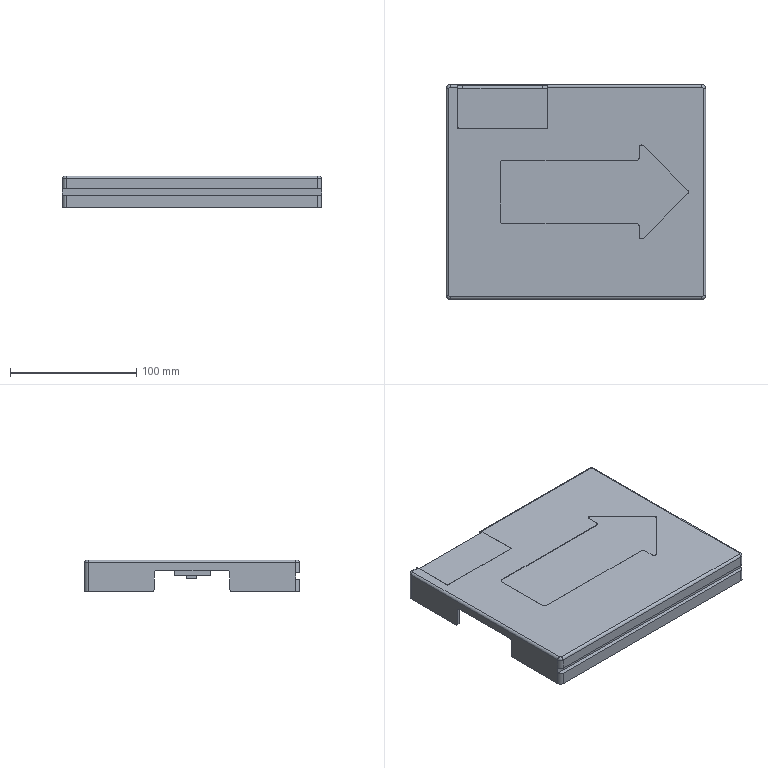NC program | NX | posted with a generic post | part box 205 x 170 x 25 mm
Lines 98 to 1305 of 17262:
(CAVITY_MILL_1 , TOOL : D10)
N188 T04 M6
N190 G54
N192 G17 G0 G90 X-109.497 Y-4.33 B0. C0. S9500 M3
N194 G43 Z30. H4
N196 Z0.513
N198 G94 G1 Z-0.988 F1000.
N200 X-103.497 Y-0.866
N202 G3 X-102.997 Y0. R1.
N204 G1 Y43.982 F3000.
N206 G2 X-103.677 Y44.075 R6.324
N208 G1 X-107.497
N210 Y45.275
N212 X-103.556
N214 G3 X-102.5 Y45.16 R5.124
N216 G1 X-100.5
N218 G3 X-95.4 Y50.272 R5.123
N220 G1 Y74.9
N222 X95.4
N224 Y30.272
N226 G3 X100.5 Y25.16 R5.125
N228 G1 X102.5
N230 G3 X103.55 Y25.275 R5.13
N232 G1 X107.497
N234 Y24.075
N236 X103.671
N238 G2 X102.997 Y23.982 R6.33
N240 G1 Y-23.982
N242 G2 X103.672 Y-24.075 R6.329
N244 G1 X107.497
N246 Y-25.275
N248 X103.551
N250 G3 X102.5 Y-25.16 R5.129
N252 G1 X100.5
N254 G3 X95.4 Y-30.272 R5.126
N256 G1 Y-68.9
N258 Y-74.9
N260 X-0.005
N262 X-95.4
N264 Y-50.272
N266 G3 X-100.5 Y-45.16 R5.106
N268 G1 X-102.5
N270 G3 X-103.558 Y-45.275 R5.122
N272 G1 X-107.497
N274 Y-44.075
N276 X-103.679
N278 G2 X-102.997 Y-43.982 R6.322
N280 G1 Y0.
N282 X-96.997
N284 Y39.734
N286 G3 X-89.4 Y50.266 R11.123
N288 G1 Y68.9
N290 X89.4
N292 Y30.265
N294 G3 X96.997 Y19.734 R11.125
N296 G1 Y-19.735
N298 G3 X89.4 Y-30.264 R11.126
N300 G1 Y-68.9
N302 X-89.4
N304 Y-50.276
N306 G3 X-96.997 Y-39.729 R11.106
N308 G1 Y0.
N310 X-90.997
N312 Y36.054
N314 G3 X-83.4 Y50.262 R17.123
N316 G1 Y62.9
N318 X83.4
N320 Y30.26
N322 G3 X90.997 Y16.055 R17.125
N324 G1 Y-16.056
N326 G3 X83.4 Y-30.258 R17.126
N328 G1 Y-62.9
N330 X-83.4
N332 Y-50.278
N334 G3 X-90.997 Y-36.047 R17.106
N336 G1 Y0.
N338 X-84.997
N340 Y33.148
N342 G3 X-77.4 Y50.258 R23.123
N344 G1 Y56.9
N346 X77.4
N348 Y30.256
N350 G3 X84.997 Y13.149 R23.125
N352 G1 Y-13.15
N354 G3 X77.4 Y-30.253 R23.126
N356 G1 Y-56.9
N358 X-77.4
N360 Y-50.28
N362 G3 X-84.997 Y-33.138 R23.106
N364 G1 Y0.
N366 X-78.997
N368 Y30.667
N370 G3 X-71.4 Y50.255 R29.123
N372 G1 Y50.9
N374 X71.4
N376 Y30.252
N378 G3 X78.997 Y10.668 R29.125
N380 G1 Y-10.669
N382 G3 X71.4 Y-30.249 R29.126
N384 G1 Y-50.9
N386 X-71.4
N388 Y-50.281
N390 G3 X-78.997 Y-30.657 R29.106
N392 G1 Y0.
N394 X-72.997
N396 Y28.467
N398 G3 X-65.815 Y44.9 R35.123
N400 G1 X65.4
N402 Y30.249
N404 G3 X72.997 Y8.468 R35.125
N406 G1 Y-8.469
N408 G3 X65.4 Y-30.245 R35.126
N410 G1 Y-44.9
N412 X-65.813
N414 G3 X-72.997 Y-28.456 R35.106
N416 G1 Y0.
N418 X-66.997
N420 Y26.469
N422 G3 X-61.007 Y38.9 R41.123
N424 G1 X59.4
N426 Y30.243
N428 G3 X66.997 Y6.47 R41.125
N430 G1 Y-6.471
N432 G3 X59.4 Y-30.242 R41.126
N434 G1 Y-38.9
N436 X-61.003
N438 G3 X-66.997 Y-26.457 R41.106
N440 G1 Y0.
N442 X-60.997
N444 Y24.626
N446 G3 X-56.723 Y32.9 R47.123
N448 G1 X53.4
N450 Y30.236
N452 G3 X60.997 Y4.627 R47.125
N454 G1 Y-4.628
N456 G3 X53.4 Y-30.235 R47.126
N458 G1 Y-32.9
N460 X-56.718
N462 G3 X-60.997 Y-24.614 R47.106
N464 G1 Y0.
N466 X-54.997
N468 Y22.907
N470 G3 X-52.823 Y26.9 R53.123
N472 G1 X47.508
N474 G3 X54.997 Y2.908 R53.125
N476 G1 Y-2.909
N478 G3 X47.508 Y-26.9 R53.126
N480 G1 X-52.817
N482 G3 X-54.997 Y-22.895 R53.106
N484 G1 Y0.
N486 X-48.997
N488 Y20.9
N490 X42.15
N492 G3 X48.997 Y1.291 R59.125
N494 G1 Y-1.292
N496 G3 X42.15 Y-20.9 R59.126
N498 G1 X-48.997
N500 Y0.
N502 X-42.997
N504 Y14.9
N506 X37.243
N508 G3 X42.87 Y-0.001 R65.125
N510 X37.244 Y-14.9 R65.126
N512 G1 X-42.997
N514 Y0.
N516 X-36.997
N518 Y8.9
N520 X32.691
N522 G3 X36.17 Y-0.001 R71.125
N524 X32.691 Y-8.9 R71.126
N526 G1 X-36.997
N528 Y0.
N530 X-30.997
N532 Y2.9
N534 X28.425
N536 G3 X29.595 Y-0.001 R77.125
N538 X28.426 Y-2.9 R77.126
N540 G1 X-30.997
N542 Y0.
N544 G3 X-31.497 Y0.866 R1.
N546 G1 Z0.513
N548 G0 X-109.497 Y-4.33 Z-0.475
N550 G1 Z-1.975 F1000.
N552 X-103.497 Y-0.866
N554 G3 X-102.997 Y0. R1.
N556 G1 Y43.729 F3000.
N558 G2 X-103.58 Y43.802 R6.284
N560 G1 X-107.497
N562 Y45.002
N564 X-103.472
N566 G3 X-102.861 Y44.923 R5.084
N568 X-100.151 Y44.92 R20.2
N570 X-95.4 Y49.997 R5.088
N572 G1 Y74.9
N574 X95.4
N576 Y29.995
N578 G3 X100.164 Y24.92 R5.085
N580 X102.829 Y24.919 R21.254
N582 X103.477 Y25.002 R5.088
N584 G1 X107.497
N586 Y24.852
N588 Y23.802
N590 X103.585
N592 G2 X102.997 Y23.728 R6.288
N594 G1 Y-23.72
N596 G2 X103.622 Y-23.801 R6.3
N598 G1 X107.497
N600 Y-25.001
N602 X103.509
N604 G3 X102.5 Y-24.9 R5.1
N606 G1 X100.5
N608 G3 X95.4 Y-30.001 R5.1
N610 G1 Y-74.9
N612 X-95.4
N614 Y-50.001
N616 G3 X-100.5 Y-44.9 R5.1
N618 G1 X-102.5
N620 G3 X-103.509 Y-45.001 R5.1
N622 G1 X-107.497
N624 Y-43.801
N626 X-103.623
N628 G2 X-102.997 Y-43.72 R6.3
N630 G1 Y0.
N632 X-96.997
N634 Y39.473
N636 G3 X-89.4 Y49.997 R11.088
N638 G1 Y68.9
N640 X89.4
N642 Y29.995
N644 G3 X96.997 Y19.473 R11.085
N646 G1 Y-19.467
N648 G3 X89.4 Y-30.002 R11.1
N650 G1 Y-68.9
N652 X-89.4
N654 Y-50.002
N656 G3 X-96.997 Y-39.467 R11.1
N658 G1 Y0.
N660 X-90.997
N662 Y35.787
N664 G3 X-83.4 Y49.997 R17.088
N666 G1 Y62.9
N668 X83.4
N670 Y29.995
N672 G3 X90.997 Y15.787 R17.085
N674 G1 Y-15.784
N676 G3 X83.4 Y-30.002 R17.1
N678 G1 Y-62.9
N680 X-83.4
N682 Y-50.001
N684 G3 X-90.997 Y-35.784 R17.1
N686 G1 Y0.
N688 X-84.997
N690 Y32.877
N692 G3 X-77.4 Y49.997 R23.088
N694 G1 Y56.9
N696 X77.4
N698 Y29.995
N700 G3 X84.997 Y12.877 R23.085
N702 G1 Y-12.875
N704 G3 X77.4 Y-30.003 R23.1
N706 G1 Y-56.9
N708 X-77.4
N710 Y-50.
N712 G3 X-84.997 Y-32.875 R23.1
N714 G1 Y0.
N716 X-78.997
N718 Y30.394
N720 G3 X-71.4 Y49.997 R29.088
N722 G1 Y50.9
N724 X71.4
N726 Y29.995
N728 G3 X78.997 Y10.394 R29.085
N730 G1 Y-10.393
N732 G3 X71.4 Y-30.003 R29.1
N734 G1 Y-50.9
N736 X-71.4
N738 Y-50.
N740 G3 X-78.997 Y-30.393 R29.1
N742 G1 Y0.
N744 X-72.997
N746 Y28.193
N748 G3 X-65.772 Y44.9 R35.088
N750 G1 X65.4
N752 Y29.995
N754 G3 X72.997 Y8.192 R35.085
N756 G1 Y-8.192
N758 G3 X65.4 Y-30.004 R35.1
N760 G1 Y-44.9
N762 X-65.773
N764 G3 X-72.997 Y-28.192 R35.1
N766 G1 Y0.
N768 X-66.997
N770 Y26.194
N772 G3 X-60.927 Y38.9 R41.088
N774 G1 X59.4
N776 Y29.995
N778 G3 X66.997 Y6.193 R41.085
N780 G1 Y-6.193
N782 G3 X59.4 Y-30.005 R41.1
N784 G1 Y-38.9
N786 X-60.927
N788 G3 X-66.997 Y-26.193 R41.1
N790 G1 Y0.
N792 X-60.997
N794 Y24.35
N796 G3 X-56.614 Y32.9 R47.088
N798 G1 X53.4
N800 Y29.995
N802 G3 X60.997 Y4.349 R47.085
N804 G1 Y-4.35
N806 G3 X53.4 Y-30.005 R47.1
N808 G1 Y-32.9
N810 X-56.614
N812 G3 X-60.997 Y-24.35 R47.1
N814 G1 Y0.
N816 X-54.997
N818 Y22.63
N820 G3 X-52.688 Y26.9 R53.088
N822 G1 X47.49
N824 G3 X54.997 Y2.629 R53.085
N826 G1 Y-2.63
N828 G3 X47.491 Y-26.9 R53.1
N830 G1 X-52.688
N832 G3 X-54.997 Y-22.63 R53.1
N834 G1 Y0.
N836 X-48.997
N838 Y20.9
N840 X42.104
N842 G3 X48.997 Y1.012 R59.085
N844 G1 Y-1.013
N846 G3 X42.105 Y-20.9 R59.1
N848 G1 X-48.997
N850 Y0.
N852 X-42.997
N854 Y14.9
N856 X37.175
N858 G3 X42.724 Y-0.001 R65.085
N860 X37.176 Y-14.9 R65.1
N862 G1 X-42.997
N864 Y0.
N866 X-36.997
N868 Y8.9
N870 X32.602
N872 G3 X36.039 Y-0.001 R71.085
N874 X32.603 Y-8.9 R71.1
N876 G1 X-36.997
N878 Y0.
N880 X-30.997
N882 Y2.9
N884 X28.319
N886 G3 X29.476 Y-0.001 R77.085
N888 X28.32 Y-2.9 R77.1
N890 G1 X-30.997
N892 Y0.
N894 G3 X-31.497 Y0.866 R1.
N896 G1 Z-0.475
N898 G0 X-109.497 Y-4.33 Z-1.463
N900 G1 Z-2.963 F1000.
N902 X-103.497 Y-0.866
N904 G3 X-102.997 Y0. R1.
N906 G1 Y43.72 F3000.
N908 G2 X-103.618 Y43.8 R6.3
N910 G1 X-107.497
N912 Y45.
N914 X-103.505
N916 G3 X-102.49 Y44.9 R5.1
N918 G1 X-100.491
N920 G3 X-95.405 Y49.775 R5.1
N922 G1 X-95.4 Y49.774
N924 Y74.9
N926 X95.4
N928 Y29.993
N930 G3 X100.501 Y24.9 R5.1
N932 G1 X102.482
N934 G3 X103.505 Y25. R5.1
N936 G1 X107.497
N938 Y23.8
N940 X103.618
N942 G2 X102.997 Y23.72 R6.3
N944 G1 Y-23.72
N946 G2 X103.618 Y-23.8 R6.3
N948 G1 X107.497
N950 Y-25.
N952 X103.505
N954 G3 X102.5 Y-24.9 R5.1
N956 G1 X100.5
N958 G3 X97.051 Y-26.243 R5.1
N960 X95.4 Y-30. R5.1
N962 G1 Y-68.9
N964 Y-74.9
N966 X-95.4
N968 Y-49.81
N970 G3 X-100.5 Y-44.9 R5.108
N972 G1 X-102.5
N974 G3 X-103.502 Y-45. R5.103
N976 G1 X-107.497
N978 Y-43.8
N980 X-103.615
N982 G2 X-102.997 Y-43.72 R6.303
N984 G1 Y0.
N986 X-96.997
N988 Y39.467
N990 G3 X-89.433 Y49.149 R11.1
N992 X-89.4 Y49.774 R6.
N994 G1 Y68.9
N996 X89.4
N998 Y29.988
N1000 G3 X96.997 Y19.467 R11.1
N1002 G1 Y-19.467
N1004 G3 X92.994 Y-21.823 R11.1
N1006 X89.4 Y-30. R11.1
N1008 G1 Y-68.9
N1010 X-89.4
N1012 Y-49.693
N1014 G3 X-96.997 Y-39.468 R11.108
N1016 G1 Y0.
N1018 X-90.997
N1020 Y35.783
N1022 G3 X-83.456 Y48.611 R17.1
N1024 X-83.4 Y49.774 R12.
N1026 G1 Y62.9
N1028 X83.4
N1030 Y29.985
N1032 G3 X90.997 Y15.783 R17.1
N1034 G1 Y-15.783
N1036 G3 X88.937 Y-17.402 R17.1
N1038 X83.4 Y-30. R17.1
N1040 G1 Y-62.9
N1042 X-83.4
N1044 X-83.402 Y-49.523
N1046 G3 X-90.997 Y-35.784 R17.108
N1048 G1 Y0.
N1050 X-84.997
N1052 Y32.875
N1054 G3 X-77.48 Y48.078 R23.1
N1056 X-77.4 Y49.774 R18.
N1058 G1 Y56.9
N1060 X77.4
N1062 Y29.98
N1064 G3 X84.997 Y12.875 R23.1
N1066 G1 Y-12.875
N1068 G3 X77.4 Y-30. R23.1
N1070 G1 Y-56.9
N1072 X-77.401
N1074 X-77.405 Y-49.353
N1076 G3 X-84.997 Y-32.875 R23.108
N1078 G1 Y0.
N1080 X-78.997
N1082 Y30.393
N1084 G3 X-71.504 Y47.546 R29.1
N1086 X-71.4 Y49.774 R24.
N1088 G1 Y50.9
N1090 X71.4
N1092 Y29.975
N1094 G3 X78.997 Y10.393 R29.1
N1096 G1 Y-10.393
N1098 G3 X71.4 Y-30. R29.1
N1100 G1 Y-50.9
N1102 X-71.404
N1104 X-71.405 Y-49.266
N1106 G3 X-78.997 Y-30.393 R29.108
N1108 G1 Y0.
N1110 X-72.997
N1112 Y28.191
N1114 G3 X-65.772 Y44.9 R35.1
N1116 G1 X65.4
N1118 Y29.97
N1120 G3 X72.997 Y8.191 R35.1
N1122 G1 Y-8.191
N1124 G3 X65.4 Y-30. R35.1
N1126 G1 Y-44.9
N1128 X-65.769
N1130 G3 X-72.997 Y-28.191 R35.108
N1132 G1 Y0.
N1134 X-66.997
N1136 Y26.193
N1138 G3 X-60.927 Y38.9 R41.1
N1140 G1 X59.4
N1142 Y29.965
N1144 G3 X66.997 Y6.193 R41.1
N1146 G1 Y-6.193
N1148 G3 X59.4 Y-30. R41.1
N1150 G1 Y-38.9
N1152 X-60.925
N1154 G3 X-66.997 Y-26.192 R41.108
N1156 G1 Y0.
N1158 X-60.997
N1160 Y24.349
N1162 G3 X-56.614 Y32.9 R47.1
N1164 G1 X53.4
N1166 Y29.959
N1168 G3 X60.997 Y4.349 R47.1
N1170 G1 Y-4.349
N1172 G3 X53.4 Y-30. R47.1
N1174 G1 Y-32.9
N1176 X-56.612
N1178 G3 X-60.997 Y-24.348 R47.108
N1180 G1 Y0.
N1182 X-54.997
N1184 Y22.63
N1186 G3 X-52.688 Y26.9 R53.1
N1188 G1 X47.491
N1190 G3 X54.997 Y2.63 R53.1
N1192 G1 Y-2.63
N1194 G3 X47.491 Y-26.9 R53.1
N1196 G1 X-52.686
N1198 G3 X-54.997 Y-22.628 R53.108
N1200 G1 Y0.
N1202 X-48.997
N1204 Y20.9
N1206 X42.105
N1208 G3 X48.997 Y1.012 R59.1
N1210 G1 Y-1.012
N1212 G3 X42.105 Y-20.9 R59.1
N1214 G1 X-48.997
N1216 Y0.
N1218 X-42.997
N1220 Y14.9
N1222 X37.175
N1224 G3 X42.724 Y0. R65.1
N1226 X37.175 Y-14.9 R65.1
N1228 G1 X-42.997
N1230 Y0.
N1232 X-36.997
N1234 Y8.9
N1236 X32.603
N1238 G3 X36.039 Y0. R71.1
N1240 X32.603 Y-8.9 R71.1
N1242 G1 X-36.997
N1244 Y0.
N1246 X-30.997
N1248 Y2.9
N1250 X28.32
N1252 G3 X29.476 Y0. R77.1
N1254 X28.32 Y-2.9 R77.1
N1256 G1 X-30.997
N1258 Y0.
N1260 G3 X-31.497 Y0.866 R1.
N1262 G1 Z-1.463
N1264 G0 X-109.498 Y-4.33 Z-2.45
N1266 G1 Z-3.95 F1000.
N1268 X-103.498 Y-0.866
N1270 G3 X-102.998 Y0. R1.
N1272 G1 Y43.72 F3000.
N1274 G2 X-103.618 Y43.8 R6.3
N1276 G1 X-107.498
N1278 Y45.
N1280 X-103.505
N1282 G3 X-102.49 Y44.9 R5.1
N1284 G1 X-100.491
N1286 G3 X-95.405 Y49.775 R5.1
N1288 G1 X-95.4 Y49.774
N1290 Y74.9
N1292 X95.4
N1294 Y29.993
N1296 G3 X100.501 Y24.9 R5.1
N1298 G1 X102.482
N1300 G3 X103.505 Y25. R5.1
N1302 G1 X107.498
N1304 Y23.8
N1306 X103.618
N1308 G2 X102.998 Y23.72 R6.3
N1310 G1 Y-23.72
N1312 G2 X103.618 Y-23.8 R6.3
N1314 G1 X107.498
N1316 Y-25.
N1318 X103.505
N1320 G3 X102.5 Y-24.9 R5.1
N1322 G1 X100.5
N1324 G3 X97.051 Y-26.243 R5.1
N1326 X95.4 Y-30. R5.1
N1328 G1 Y-68.9
N1330 Y-74.9
N1332 X-95.4
N1334 Y-49.81
N1336 G3 X-100.5 Y-44.9 R5.107
N1338 G1 X-102.5
N1340 G3 X-103.502 Y-45. R5.103
N1342 G1 X-107.498
N1344 Y-43.8
N1346 X-103.615
N1348 G2 X-102.998 Y-43.72 R6.303
N1350 G1 Y0.
N1352 X-96.998
N1354 Y39.467
N1356 G3 X-89.433 Y49.149 R11.1
N1358 X-89.4 Y49.774 R6.
N1360 G1 Y68.9
N1362 X89.4
N1364 Y29.988
N1366 G3 X96.998 Y19.467 R11.1
N1368 G1 Y-19.467
N1370 G3 X92.994 Y-21.823 R11.1
N1372 X89.4 Y-30. R11.1
N1374 G1 Y-68.9
N1376 X-89.4
N1378 Y-49.693
N1380 G3 X-96.998 Y-39.468 R11.107
N1382 G1 Y0.
N1384 X-90.998
N1386 Y35.783
N1388 G3 X-83.456 Y48.611 R17.1
N1390 X-83.4 Y49.774 R12.
N1392 G1 Y62.9
N1394 X83.4
N1396 Y29.985
N1398 G3 X90.998 Y15.783 R17.1
N1400 G1 Y-15.783
N1402 G3 X88.937 Y-17.402 R17.1
N1404 X83.4 Y-30. R17.1
N1406 G1 Y-62.9
N1408 X-83.4
N1410 X-83.402 Y-49.524
N1412 G3 X-90.998 Y-35.784 R17.107
N1414 G1 Y0.
N1416 X-84.998
N1418 Y32.874
N1420 G3 X-77.48 Y48.078 R23.1
N1422 X-77.4 Y49.774 R18.
N1424 G1 Y56.9
N1426 X77.4
N1428 Y29.98
N1430 G3 X84.998 Y12.874 R23.1
N1432 G1 Y-12.874
N1434 G3 X77.4 Y-30. R23.1
N1436 G1 Y-56.9
N1438 X-77.401
N1440 X-77.402 Y-49.438
N1442 G3 X-84.998 Y-32.875 R23.107
N1444 G1 Y0.
N1446 X-78.998
N1448 Y30.392
N1450 G3 X-71.504 Y47.546 R29.1
N1452 X-71.4 Y49.774 R24.
N1454 G1 Y50.9
N1456 X71.4
N1458 Y29.975
N1460 G3 X78.998 Y10.392 R29.1
N1462 G1 Y-10.392
N1464 G3 X71.4 Y-30. R29.1
N1466 G1 Y-50.9
N1468 X-71.402
N1470 Y-49.364
N1472 G3 X-78.998 Y-30.392 R29.107
N1474 G1 Y0.
N1476 X-72.998
N1478 Y28.191
N1480 G3 X-65.772 Y44.9 R35.1
N1482 G1 X65.4
N1484 Y29.97
N1486 G3 X72.998 Y8.191 R35.1
N1488 G1 Y-8.191
N1490 G3 X65.4 Y-30. R35.1
N1492 G1 Y-44.9
N1494 X-65.769
N1496 G3 X-72.998 Y-28.191 R35.107
N1498 G1 Y0.
N1500 X-66.998
N1502 Y26.193
N1504 G3 X-60.927 Y38.9 R41.1
N1506 G1 X59.4
N1508 Y29.965
N1510 G3 X66.998 Y6.193 R41.1
N1512 G1 Y-6.193
N1514 G3 X59.4 Y-30. R41.1
N1516 G1 Y-38.9
N1518 X-60.925
N1520 G3 X-66.998 Y-26.191 R41.107
N1522 G1 Y0.
N1524 X-60.998
N1526 Y24.349
N1528 G3 X-56.614 Y32.9 R47.1
N1530 G1 X53.4
N1532 Y29.959
N1534 G3 X60.998 Y4.349 R47.1
N1536 G1 Y-4.349
N1538 G3 X53.4 Y-30. R47.1
N1540 G1 Y-32.9
N1542 X-56.612
N1544 G3 X-60.998 Y-24.348 R47.107
N1546 G1 Y0.
N1548 X-54.998
N1550 Y22.63
N1552 G3 X-52.688 Y26.9 R53.1
N1554 G1 X47.491
N1556 G3 X54.998 Y2.63 R53.1
N1558 G1 Y-2.63
N1560 G3 X47.491 Y-26.9 R53.1
N1562 G1 X-52.686
N1564 G3 X-54.998 Y-22.628 R53.107
N1566 G1 Y0.
N1568 X-48.998
N1570 Y20.9
N1572 X42.105
N1574 G3 X48.998 Y1.012 R59.1
N1576 G1 Y-1.012
N1578 G3 X42.105 Y-20.9 R59.1
N1580 G1 X-48.998
N1582 Y0.
N1584 X-42.998
N1586 Y14.9
N1588 X37.175
N1590 G3 X42.724 Y0. R65.1
N1592 X37.175 Y-14.9 R65.1
N1594 G1 X-42.998
N1596 Y0.
N1598 X-36.998
N1600 Y8.9
N1602 X32.603
N1604 G3 X36.039 Y0. R71.1
N1606 X32.603 Y-8.9 R71.1
N1608 G1 X-36.998
N1610 Y0.
N1612 X-30.998
N1614 Y2.9
N1616 X28.32
N1618 G3 X29.476 Y0. R77.1
N1620 X28.32 Y-2.9 R77.1
N1622 G1 X-30.998
N1624 Y0.
N1626 G3 X-31.498 Y0.866 R1.
N1628 G1 Z-2.45
N1630 G0 X-109.498 Y-4.33 Z-3.438
N1632 G1 Z-4.938 F1000.
N1634 X-103.498 Y-0.866
N1636 G3 X-102.998 Y0. R1.
N1638 G1 Y43.72 F3000.
N1640 G2 X-103.618 Y43.8 R6.3
N1642 G1 X-107.498
N1644 Y45.
N1646 X-103.505
N1648 G3 X-102.49 Y44.9 R5.1
N1650 G1 X-100.491
N1652 G3 X-95.405 Y49.775 R5.1
N1654 G1 X-95.4 Y49.774
N1656 Y74.9
N1658 X95.4
N1660 Y29.988
N1662 G3 X100.501 Y24.9 R5.1
N1664 G1 X102.482
N1666 G3 X103.505 Y25. R5.1
N1668 G1 X107.498
N1670 Y23.8
N1672 X103.618
N1674 G2 X102.998 Y23.72 R6.3
N1676 G1 Y-23.72
N1678 G2 X103.618 Y-23.8 R6.3
N1680 G1 X107.498
N1682 Y-25.
N1684 X103.505
N1686 G3 X102.5 Y-24.9 R5.1
N1688 G1 X100.5
N1690 G3 X97.051 Y-26.243 R5.1
N1692 X95.4 Y-30. R5.1
N1694 G1 Y-68.9
N1696 Y-74.9
N1698 X-95.4
N1700 Y-49.81
N1702 G3 X-100.5 Y-44.9 R5.107
N1704 G1 X-102.5
N1706 G3 X-103.502 Y-45. R5.103
N1708 G1 X-107.498
N1710 Y-43.8
N1712 X-103.615
N1714 G2 X-102.998 Y-43.72 R6.303
N1716 G1 Y0.
N1718 X-96.998
N1720 Y39.467
N1722 G3 X-89.433 Y49.149 R11.1
N1724 X-89.4 Y49.774 R6.
N1726 G1 Y68.9
N1728 X89.4
N1730 Y29.988
N1732 G3 X96.998 Y19.467 R11.1
N1734 G1 Y-19.467
N1736 G3 X92.994 Y-21.823 R11.1
N1738 X89.4 Y-30. R11.1
N1740 G1 Y-68.9
N1742 X-89.4
N1744 X-89.404 Y-49.578
N1746 G3 X-96.998 Y-39.468 R11.107
N1748 G1 Y0.
N1750 X-90.998
N1752 Y35.783
N1754 G3 X-83.456 Y48.611 R17.1
N1756 X-83.4 Y49.774 R12.
N1758 G1 Y62.9
N1760 X83.4
N1762 Y29.985
N1764 G3 X90.998 Y15.783 R17.1
N1766 G1 Y-15.783
N1768 G3 X88.937 Y-17.402 R17.1
N1770 X83.4 Y-30. R17.1
N1772 G1 Y-62.9
N1774 X-83.401
N1776 X-83.409 Y-49.346
N1778 G3 X-90.998 Y-35.784 R17.107
N1780 G1 Y0.
N1782 X-84.998
N1784 Y32.874
N1786 G3 X-77.48 Y48.078 R23.1
N1788 X-77.4 Y49.774 R18.
N1790 G1 Y56.9
N1792 X77.4
N1794 Y29.98
N1796 G3 X84.998 Y12.874 R23.1
N1798 G1 Y-12.874
N1800 G3 X77.4 Y-30. R23.1
N1802 G1 Y-56.9
N1804 X-77.405
N1806 X-77.409 Y-49.228
N1808 G3 X-84.998 Y-32.875 R23.107
N1810 G1 Y0.
N1812 X-78.998
N1814 Y30.392
N1816 G3 X-71.504 Y47.546 R29.1
N1818 X-71.4 Y49.774 R24.
N1820 G1 Y50.9
N1822 X71.4
N1824 Y29.975
N1826 G3 X78.998 Y10.392 R29.1
N1828 G1 Y-10.392
N1830 G3 X71.4 Y-30. R29.1
N1832 G1 Y-50.9
N1834 X-71.408
N1836 X-71.412 Y-49.026
N1838 G3 X-78.998 Y-30.392 R29.107
N1840 G1 Y0.
N1842 X-72.998
N1844 Y28.191
N1846 G3 X-65.772 Y44.9 R35.1
N1848 G1 X65.4
N1850 Y29.97
N1852 G3 X72.998 Y8.191 R35.1
N1854 G1 Y-8.191
N1856 G3 X65.4 Y-30. R35.1
N1858 G1 Y-44.9
N1860 X-65.769
N1862 G3 X-72.998 Y-28.191 R35.107
N1864 G1 Y0.
N1866 X-66.998
N1868 Y26.192
N1870 G3 X-60.927 Y38.9 R41.1
N1872 G1 X59.4
N1874 Y29.965
N1876 G3 X66.998 Y6.192 R41.1
N1878 G1 Y-6.192
N1880 G3 X59.4 Y-30. R41.1
N1882 G1 Y-38.9
N1884 X-60.925
N1886 G3 X-66.998 Y-26.192 R41.107
N1888 G1 Y0.
N1890 X-60.998
N1892 Y24.349
N1894 G3 X-56.614 Y32.9 R47.1
N1896 G1 X53.4
N1898 Y29.959
N1900 G3 X60.998 Y4.349 R47.1
N1902 G1 Y-4.349
N1904 G3 X53.4 Y-30. R47.1
N1906 G1 Y-32.9
N1908 X-56.612
N1910 G3 X-60.998 Y-24.348 R47.107
N1912 G1 Y0.
N1914 X-54.998
N1916 Y22.629
N1918 G3 X-52.688 Y26.9 R53.1
N1920 G1 X47.491
N1922 G3 X54.998 Y2.629 R53.1
N1924 G1 Y-2.629
N1926 G3 X47.491 Y-26.9 R53.1
N1928 G1 X-52.687
N1930 G3 X-54.998 Y-22.628 R53.107
N1932 G1 Y0.
N1934 X-48.998
N1936 Y20.9
N1938 X42.105
N1940 G3 X48.998 Y1.012 R59.1
N1942 G1 Y-1.012
N1944 G3 X42.105 Y-20.9 R59.1
N1946 G1 X-48.998
N1948 Y0.
N1950 X-42.998
N1952 Y14.9
N1954 X37.175
N1956 G3 X42.724 Y0. R65.1
N1958 X37.175 Y-14.9 R65.1
N1960 G1 X-42.998
N1962 Y0.
N1964 X-36.998
N1966 Y8.9
N1968 X32.603
N1970 G3 X36.039 Y0. R71.1
N1972 X32.603 Y-8.9 R71.1
N1974 G1 X-36.998
N1976 Y0.
N1978 X-30.998
N1980 Y2.9
N1982 X28.32
N1984 G3 X29.476 Y0. R77.1
N1986 X28.32 Y-2.9 R77.1
N1988 G1 X-30.998
N1990 Y0.
N1992 G3 X-31.498 Y0.866 R1.
N1994 G1 Z-3.438
N1996 G0 X-109.498 Y-4.33 Z-4.425
N1998 G1 Z-5.925 F1000.
N2000 X-103.498 Y-0.866
N2002 G3 X-102.998 Y0. R1.
N2004 G1 Y43.72 F3000.
N2006 G2 X-103.618 Y43.8 R6.3
N2008 G1 X-107.498
N2010 Y45.
N2012 X-103.505
N2014 G3 X-102.49 Y44.9 R5.1
N2016 G1 X-100.491
N2018 G3 X-95.405 Y49.775 R5.1
N2020 G1 X-95.4 Y49.774
N2022 Y74.9
N2024 X95.4
N2026 Y29.993
N2028 G3 X100.501 Y24.9 R5.1
N2030 G1 X102.482
N2032 G3 X103.505 Y25. R5.1
N2034 G1 X107.498
N2036 Y23.8
N2038 X103.618
N2040 G2 X102.998 Y23.72 R6.3
N2042 G1 Y-23.72
N2044 G2 X103.618 Y-23.8 R6.3
N2046 G1 X107.498
N2048 Y-25.
N2050 X103.505
N2052 G3 X102.5 Y-24.9 R5.1
N2054 G1 X100.5
N2056 G3 X97.051 Y-26.243 R5.1
N2058 X95.4 Y-30. R5.1
N2060 G1 Y-68.9
N2062 Y-74.9
N2064 X-95.4
N2066 Y-49.81
N2068 G3 X-100.5 Y-44.9 R5.107
N2070 G1 X-102.5
N2072 G3 X-103.502 Y-45. R5.103
N2074 G1 X-107.498
N2076 Y-43.8
N2078 X-103.615
N2080 G2 X-102.998 Y-43.72 R6.303
N2082 G1 Y0.
N2084 X-96.998
N2086 Y39.467
N2088 G3 X-89.433 Y49.149 R11.1
N2090 X-89.4 Y49.774 R6.
N2092 G1 Y68.9
N2094 X89.4
N2096 Y29.988
N2098 G3 X96.998 Y19.467 R11.1
N2100 G1 Y-19.467
N2102 G3 X92.994 Y-21.823 R11.1
N2104 X89.4 Y-30. R11.1
N2106 G1 Y-68.9
N2108 X-89.4
N2110 Y-49.694
N2112 G3 X-96.998 Y-39.468 R11.107
N2114 G1 Y0.
N2116 X-90.998
N2118 Y35.783
N2120 G3 X-83.456 Y48.611 R17.1
N2122 X-83.4 Y49.774 R12.
N2124 G1 Y62.9
N2126 X83.4
N2128 Y29.985
N2130 G3 X90.998 Y15.783 R17.1
N2132 G1 Y-15.783
N2134 G3 X88.937 Y-17.402 R17.1
N2136 X83.4 Y-30. R17.1
N2138 G1 Y-62.9
N2140 X-83.4
N2142 Y-49.609
N2144 G3 X-90.998 Y-35.784 R17.107
N2146 G1 Y0.
N2148 X-84.998
N2150 Y32.874
N2152 G3 X-77.48 Y48.078 R23.1
N2154 X-77.4 Y49.774 R18.
N2156 G1 Y56.9
N2158 X77.4
N2160 Y29.98
N2162 G3 X84.998 Y12.874 R23.1
N2164 G1 Y-12.874
N2166 G3 X77.4 Y-30. R23.1
N2168 G1 Y-56.9
N2170 X-77.4
N2172 Y-49.54
N2174 G3 X-84.998 Y-32.874 R23.107
N2176 G1 Y0.
N2178 X-78.998
N2180 Y30.392
N2182 G3 X-71.504 Y47.546 R29.1
N2184 X-71.4 Y49.774 R24.
N2186 G1 Y50.9
N2188 X71.4
N2190 Y29.975
N2192 G3 X78.998 Y10.392 R29.1
N2194 G1 Y-10.392
N2196 G3 X71.4 Y-30. R29.1
N2198 G1 Y-50.9
N2200 X-71.4
N2202 Y-49.479
N2204 G3 X-78.998 Y-30.392 R29.107
N2206 G1 Y0.
N2208 X-72.998
N2210 Y28.191
N2212 G3 X-65.772 Y44.9 R35.1
N2214 G1 X65.4
N2216 Y29.97
N2218 G3 X72.998 Y8.191 R35.1
N2220 G1 Y-8.191
N2222 G3 X65.4 Y-30. R35.1
N2224 G1 Y-44.9
N2226 X-65.769
N2228 G3 X-72.998 Y-28.19 R35.107
N2230 G1 Y0.
N2232 X-66.998
N2234 Y26.192
N2236 G3 X-60.927 Y38.9 R41.1
N2238 G1 X59.4
N2240 Y29.965
N2242 G3 X66.998 Y6.192 R41.1
N2244 G1 Y-6.192
N2246 G3 X59.4 Y-30. R41.1
N2248 G1 Y-38.9
N2250 X-60.924
N2252 G3 X-66.998 Y-26.19 R41.107
N2254 G1 Y0.
N2256 X-60.998
N2258 Y24.349
N2260 G3 X-56.614 Y32.9 R47.1
N2262 G1 X53.4
N2264 Y29.959
N2266 G3 X60.998 Y4.349 R47.1
N2268 G1 Y-4.349
N2270 G3 X53.4 Y-30. R47.1
N2272 G1 Y-32.9
N2274 X-56.611
N2276 G3 X-60.998 Y-24.347 R47.107
N2278 G1 Y0.
N2280 X-54.998
N2282 Y22.629
N2284 G3 X-52.688 Y26.9 R53.1
N2286 G1 X47.491
N2288 G3 X54.998 Y2.629 R53.1
N2290 G1 Y-2.629
N2292 G3 X47.491 Y-26.9 R53.1
N2294 G1 X-52.686
N2296 G3 X-54.998 Y-22.627 R53.107
N2298 G1 Y0.
N2300 X-48.998
N2302 Y20.9
N2304 X42.105
N2306 G3 X48.998 Y1.012 R59.1
N2308 G1 Y-1.012
N2310 G3 X42.105 Y-20.9 R59.1
N2312 G1 X-48.998
N2314 Y0.
N2316 X-42.998
N2318 Y14.9
N2320 X37.175
N2322 G3 X42.724 Y0. R65.1
N2324 X37.175 Y-14.9 R65.1
N2326 G1 X-42.998
N2328 Y0.
N2330 X-36.998
N2332 Y8.9
N2334 X32.603
N2336 G3 X36.039 Y0. R71.1
N2338 X32.603 Y-8.9 R71.1
N2340 G1 X-36.998
N2342 Y0.
N2344 X-30.998
N2346 Y2.9
N2348 X28.32
N2350 G3 X29.476 Y0. R77.1
N2352 X28.32 Y-2.9 R77.1
N2354 G1 X-30.998
N2356 Y0.
N2358 G3 X-31.498 Y0.866 R1.
N2360 G1 Z-4.425
N2362 G0 X-109.498 Y-4.33 Z-5.413
N2364 G1 Z-6.913 F1000.
N2366 X-103.498 Y-0.866
N2368 G3 X-102.998 Y0. R1.
N2370 G1 Y43.72 F3000.
N2372 G2 X-103.618 Y43.8 R6.3
N2374 G1 X-107.498
N2376 Y45.
N2378 X-103.505
N2380 G3 X-102.49 Y44.9 R5.1
N2382 G1 X-100.491
N2384 G3 X-95.405 Y49.775 R5.1
N2386 G1 X-95.4 Y49.774
N2388 Y74.9
N2390 X95.4
N2392 Y29.993
N2394 G3 X100.501 Y24.9 R5.1
N2396 G1 X102.482
N2398 G3 X103.505 Y25. R5.1
N2400 G1 X107.498
N2402 Y23.8
N2404 X103.618
N2406 G2 X102.998 Y23.72 R6.3
N2408 G1 Y-23.72
N2410 G2 X103.618 Y-23.8 R6.3
N2412 G1 X107.498
N2414 Y-25.
N2416 X103.505
N2418 G3 X102.5 Y-24.9 R5.1
N2420 G1 X100.5
N2422 G3 X97.051 Y-26.243 R5.1
N2424 X95.4 Y-30. R5.1
N2426 G1 Y-68.9
N2428 Y-74.9
N2430 X-95.4
N2432 Y-49.81
N2434 G3 X-100.5 Y-44.9 R5.106
N2436 G1 X-102.5
N2438 G3 X-103.502 Y-45. R5.103
N2440 G1 X-107.498
N2442 Y-43.8
N2444 X-103.615
N2446 G2 X-102.998 Y-43.72 R6.303
N2448 G1 Y0.
N2450 X-96.998
N2452 Y39.467
N2454 G3 X-89.433 Y49.149 R11.1
N2456 X-89.4 Y49.774 R6.
N2458 G1 Y68.9
N2460 X89.4
N2462 Y29.988
N2464 G3 X96.998 Y19.467 R11.1
N2466 G1 Y-19.467
N2468 G3 X92.994 Y-21.823 R11.1
N2470 X89.4 Y-30. R11.1
N2472 G1 Y-68.9
N2474 X-89.4
N2476 X-89.404 Y-49.579
N2478 G3 X-96.998 Y-39.467 R11.106
N2480 G1 Y0.
N2482 X-90.998
N2484 Y35.783
N2486 G3 X-83.456 Y48.611 R17.1
N2488 X-83.4 Y49.774 R12.
N2490 G1 Y62.9
N2492 X83.4
N2494 Y29.985
N2496 G3 X90.998 Y15.783 R17.1
N2498 G1 Y-15.783
N2500 G3 X88.937 Y-17.402 R17.1
N2502 X83.4 Y-30. R17.1
N2504 G1 Y-62.9
N2506 X-83.401
N2508 X-83.404 Y-49.462
N2510 G3 X-84.042 Y-45.35 R17.106
N2512 X-90.998 Y-35.783 R17.106
N2514 G1 Y0.
N2516 X-84.998
N2518 Y32.874
N2520 G3 X-77.48 Y48.078 R23.1
N2522 X-77.4 Y49.774 R18.
N2524 G1 Y56.9
N2526 X77.4
N2528 Y29.98
N2530 G3 X84.998 Y12.874 R23.1
N2532 G1 Y-12.874
N2534 G3 X77.4 Y-30. R23.1
N2536 G1 Y-56.9
N2538 X-77.403
N2540 X-77.404 Y-49.366
N2542 G3 X-78.269 Y-43.716 R23.106
N2544 X-84.998 Y-32.874 R23.106
N2546 G1 Y0.
N2548 X-78.998
N2550 Y30.392
N2552 G3 X-71.504 Y47.546 R29.1
N2554 X-71.4 Y49.774 R24.
N2556 G1 Y50.9
N2558 X71.4
N2560 Y29.975
N2562 G3 X78.998 Y10.392 R29.1
N2564 G1 Y-10.392
N2566 G3 X71.4 Y-30. R29.1
N2568 G1 Y-50.9
N2570 X-71.404
N2572 X-71.405 Y-49.282
N2574 G3 X-72.496 Y-42.082 R29.106
N2576 X-78.998 Y-30.392 R29.106
N2578 G1 Y0.
N2580 X-72.998
N2582 Y28.191
N2584 G3 X-65.772 Y44.9 R35.1
N2586 G1 X65.4
N2588 Y29.97
N2590 G3 X72.998 Y8.191 R35.1
N2592 G1 Y-8.191
N2594 G3 X65.4 Y-30. R35.1
N2596 G1 Y-44.9